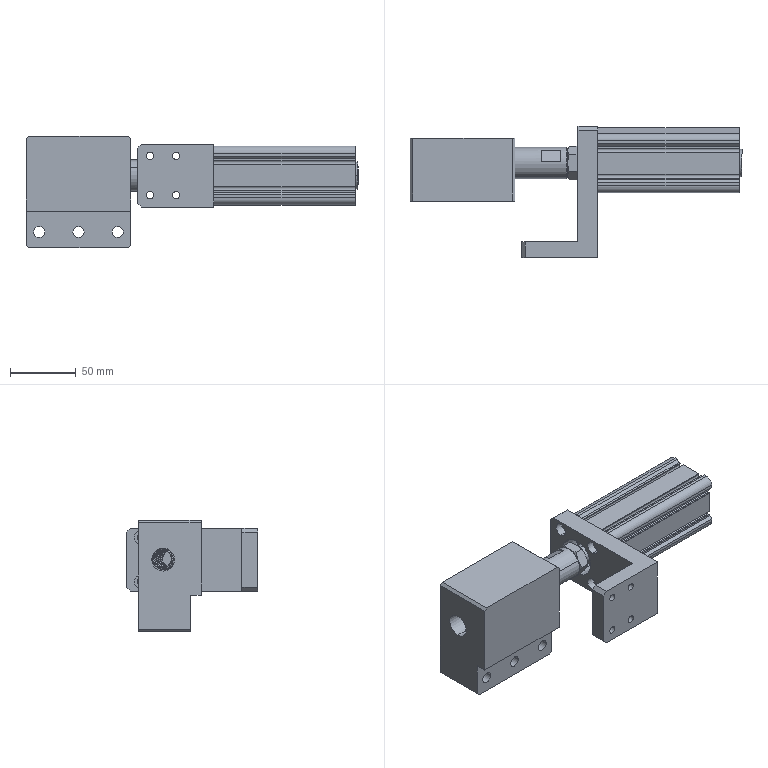Part | SolidWorks | 9 solids | 364 faces | box 253.005 x 100 x 85 mm | volume 494413 mm3 | plane 168 | cylinder 142 | cone 48 | spline 6 | commonest cylinder face diameters 4.26 x18 4.917 x16 0.6 x8 5.5 x8 5.6 x8 6 x8